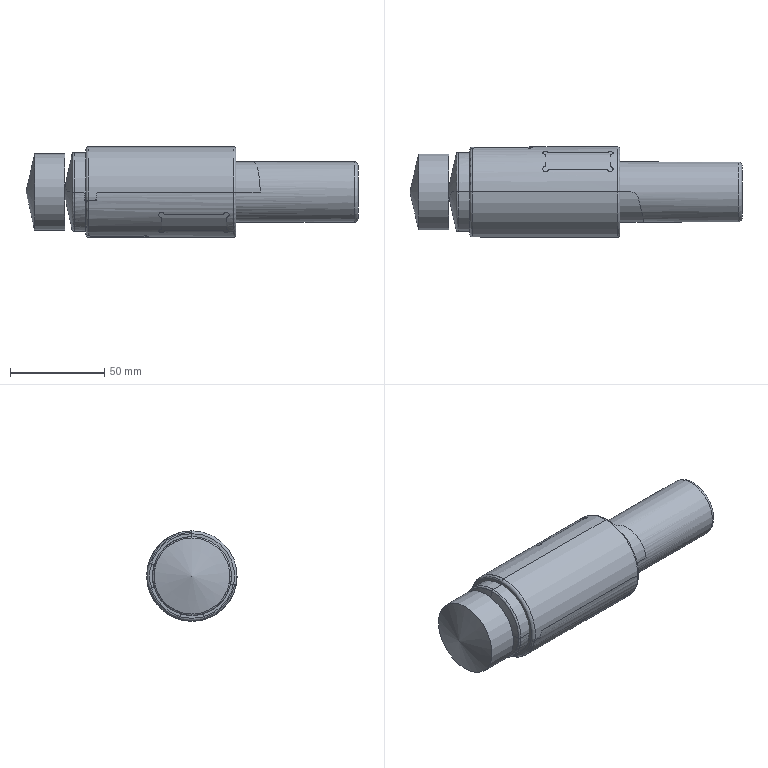NC program | NX | posted with a generic post | part box 176.413 x 48 x 48 mm
Lines 2819 to 3940 of 71815:
(ZLEVEL_PROFILE_COPY_COPY_COPY , TOOL : D6)
N5612 T06 M6
N5614 G54
N5616 G18 G0 G90 X-130.33 Z1.925 S3800 M3
N5618 G43 Y34.947 H6
N5620 Y25.5
N5622 G94 G1 X-115.85 Y24.741 F1000.
N5624 Y24.539 Z-1.925
N5626 X-128.05 Y23.9
N5628 X-140.25 F1600.
N5630 Z1.925
N5632 X-115.85
N5634 Z-1.925
N5636 X-128.05
N5638 X-133.779 Y23.8
N5640 X-140.25
N5642 Z1.925
N5644 X-115.85
N5646 Z-1.925
N5648 X-128.05
N5650 X-133.779 Y23.7
N5652 X-140.25
N5654 Z1.925
N5656 X-115.85
N5658 Z-1.925
N5660 X-128.05
N5662 X-133.779 Y23.6
N5664 X-140.25
N5666 Z1.925
N5668 X-115.85
N5670 Z-1.925
N5672 X-128.05
N5674 X-133.779 Y23.5
N5676 X-140.25
N5678 Z1.925
N5680 X-115.85
N5682 Z-1.925
N5684 X-128.05
N5686 X-133.779 Y23.4
N5688 X-140.25
N5690 Z1.925
N5692 X-115.85
N5694 Z-1.925
N5696 X-128.05
N5698 X-133.779 Y23.3
N5700 X-140.25
N5702 Z1.925
N5704 X-115.85
N5706 Z-1.925
N5708 X-128.05
N5710 X-133.779 Y23.2
N5712 X-140.25
N5714 Z1.925
N5716 X-115.85
N5718 Z-1.925
N5720 X-128.05
N5722 X-133.779 Y23.1
N5724 X-140.25
N5726 Z1.925
N5728 X-115.85
N5730 Z-1.925
N5732 X-128.05
N5734 X-133.779 Y23.
N5736 X-140.25
N5738 Z1.925
N5740 X-115.85
N5742 Z-1.925
N5744 X-128.05
N5746 X-133.779 Y22.9
N5748 X-140.25
N5750 Z1.925
N5752 X-115.85
N5754 Z-1.925
N5756 X-128.05
N5758 X-133.779 Y22.8
N5760 X-140.25
N5762 Z1.925
N5764 X-115.85
N5766 Z-1.925
N5768 X-128.05
N5770 X-133.779 Y22.7
N5772 X-140.25
N5774 Z1.925
N5776 X-115.85
N5778 Z-1.925
N5780 X-128.05
N5782 X-133.779 Y22.6
N5784 X-140.25
N5786 Z1.925
N5788 X-115.85
N5790 Z-1.925
N5792 X-128.05
N5794 X-133.779 Y22.5
N5796 X-140.25
N5798 Z1.925
N5800 X-115.85
N5802 Z-1.925
N5804 X-128.05
N5806 X-133.779 Y22.4
N5808 X-140.25
N5810 Z1.925
N5812 X-115.85
N5814 Z-1.925
N5816 X-128.05
N5818 X-133.779 Y22.3
N5820 X-140.25
N5822 Z1.925
N5824 X-115.85
N5826 Z-1.925
N5828 X-128.05
N5830 X-133.779 Y22.2
N5832 X-140.25
N5834 Z1.925
N5836 X-115.85
N5838 Z-1.925
N5840 X-128.05
N5842 X-133.779 Y22.1
N5844 X-140.25
N5846 Z1.925
N5848 X-115.85
N5850 Z-1.925
N5852 X-128.05
N5854 X-133.779 Y22.
N5856 X-140.25
N5858 Z1.925
N5860 X-115.85
N5862 Z-1.925
N5864 X-128.05
N5866 X-133.779 Y21.9
N5868 X-140.25
N5870 Z1.925
N5872 X-115.85
N5874 Z-1.925
N5876 X-128.05
N5878 X-133.779 Y21.8
N5880 X-140.25
N5882 Z1.925
N5884 X-115.85
N5886 Z-1.925
N5888 X-128.05
N5890 X-133.779 Y21.7
N5892 X-140.25
N5894 Z1.925
N5896 X-115.85
N5898 Z-1.925
N5900 X-128.05
N5902 X-133.779 Y21.6
N5904 X-140.25
N5906 Z1.925
N5908 X-115.85
N5910 Z-1.925
N5912 X-128.05
N5914 X-133.779 Y21.5
N5916 X-140.25
N5918 Z1.925
N5920 X-115.85
N5922 Z-1.925
N5924 X-128.05
N5926 X-133.779 Y21.4
N5928 X-140.25
N5930 Z1.925
N5932 X-115.85
N5934 Z-1.925
N5936 X-128.05
N5938 X-133.779 Y21.3
N5940 X-140.25
N5942 Z1.925
N5944 X-115.85
N5946 Z-1.925
N5948 X-128.05
N5950 X-133.779 Y21.2
N5952 X-140.25
N5954 Z1.925
N5956 X-115.85
N5958 Z-1.925
N5960 X-128.05
N5962 X-133.779 Y21.1
N5964 X-140.25
N5966 Z1.925
N5968 X-115.85
N5970 Z-1.925
N5972 X-128.05
N5974 X-133.779 Y21.
N5976 X-140.25
N5978 Z1.925
N5980 X-115.85
N5982 Z-1.925
N5984 X-128.05
N5986 X-133.779 Y20.9
N5988 X-140.25
N5990 Z1.925
N5992 X-115.85
N5994 Z-1.925
N5996 X-128.05
N5998 X-133.779 Y20.8
N6000 X-140.25
N6002 Z1.925
N6004 X-115.85
N6006 Z-1.925
N6008 X-128.05
N6010 X-133.779 Y20.7
N6012 X-140.25
N6014 Z1.925
N6016 X-115.85
N6018 Z-1.925
N6020 X-128.05
N6022 X-133.779 Y20.6
N6024 X-140.25
N6026 Z1.925
N6028 X-115.85
N6030 Z-1.925
N6032 X-128.05
N6034 X-133.779 Y20.5
N6036 X-140.25
N6038 Z1.925
N6040 X-115.85
N6042 Z-1.925
N6044 X-133.779
N6046 Y22.
N6048 G0 Y34.947
(ZLEVEL_PROFILE_COPY_1 , TOOL : D6)
N6050 X-147.954 Z2.204 S4000
N6052 Y34.931
N6054 Y24.899
N6056 G1 Y23.899 F1500.
N6058 X-147.781 Z2.5
N6060 G3 X-147.259 Z2.796 R0.6
N6062 G1 X-146.879 Z2.793
N6064 X-146.358 Z2.567
N6066 G2 X-143.955 Z2.729 R3.092
N6068 X-141.804 Z1.925 R3.246
N6070 G1 X-115.85
N6072 Z-1.925
N6074 X-141.881
N6076 G2 X-144.629 Z-3.652 R3.1
N6078 G1 X-144.645 Z-3.723
N6080 X-144.735 Z-3.757
N6082 X-145.035 Z-3.903
N6084 X-145.631 Z-4.254
N6086 X-145.997 Z-4.437
N6088 G2 X-147.12 Z-5.322 R4.283
N6090 G3 X-147.691 Z-5.505 R0.6
N6092 G1 X-148.003 Z-5.438
N6094 Y24.899
N6096 G0 X-147.958 Y24.8 Z2.204
N6098 G1 Y23.8
N6100 X-147.782 Z2.502
N6102 G3 X-147.259 Z2.797 R0.6
N6104 G1 X-146.879 Z2.793
N6106 X-146.358 Z2.567
N6108 G2 X-143.955 Z2.729 R3.092
N6110 X-141.804 Z1.925 R3.246
N6112 G1 X-115.85
N6114 Z-1.925
N6116 X-141.881
N6118 G2 X-144.627 Z-3.648 R3.1
N6120 G3 X-144.991 Z-3.846 R0.725
N6122 G1 X-146.106 Z-4.469
N6124 G2 X-147.167 Z-5.321 R4.085
N6126 G3 X-147.737 Z-5.51 R0.6
N6128 G1 X-148.058 Z-5.444
N6130 Y24.8
N6132 G0 X-147.961 Y24.7 Z2.198
N6134 G1 Y23.7
N6136 X-147.782 Z2.502
N6138 G3 X-147.259 Z2.797 R0.6
N6140 G1 X-146.879 Z2.793
N6142 X-146.358 Z2.567
N6144 G2 X-143.955 Z2.729 R3.093
N6146 X-141.804 Z1.925 R3.246
N6148 G1 X-115.85
N6150 Z-1.925
N6152 X-141.881
N6154 G2 X-144.627 Z-3.648 R3.1
N6156 X-146.568 Z-4.733 R16.601
N6158 G1 X-147.215 Z-5.32
N6160 G3 X-147.801 Z-5.448 R0.6
N6162 G1 X-148.052 Z-5.367
N6164 Y24.7
N6166 G0 X-147.958 Y24.6 Z2.203
N6168 G1 Y23.6
N6170 X-147.781 Z2.5
N6172 G3 X-147.257 Z2.793 R0.6
N6174 G1 X-146.861 Z2.787
N6176 X-146.358 Z2.567
N6178 G2 X-143.955 Z2.729 R3.099
N6180 X-141.804 Z1.925 R3.246
N6182 G1 X-115.85
N6184 Z-1.925
N6186 X-141.881
N6188 G2 X-144.635 Z-3.635 R3.153
N6190 X-145.929 Z-4.322 R6.532
N6192 X-147.262 Z-5.32 R4.227
N6194 G3 X-147.832 Z-5.507 R0.6
N6196 G1 X-148.154 Z-5.439
N6198 Y24.6
N6200 G0 X-147.958 Y24.5 Z2.203
N6202 G1 Y23.5
N6204 X-147.781 Z2.5
N6206 G3 X-147.257 Z2.793 R0.6
N6208 G1 X-146.861 Z2.787
N6210 X-146.358 Z2.566
N6212 G2 X-143.954 Z2.729 R3.1
N6214 X-141.804 Z1.925 R3.245
N6216 G1 X-115.85
N6218 Z-1.925
N6220 X-141.881
N6222 G2 X-144.606 Z-3.592 R3.126
N6224 X-145.957 Z-4.308 R5.848
N6226 X-147.309 Z-5.319 R4.307
N6228 G3 X-147.88 Z-5.505 R0.6
N6230 G1 X-148.203 Z-5.437
N6232 Y24.5
N6234 G0 X-147.959 Y24.401 Z2.203
N6236 G1 Y23.401
N6238 X-147.781 Z2.5
N6240 G3 X-147.257 Z2.793 R0.6
N6242 G1 X-146.861 Z2.787
N6244 X-146.358 Z2.566
N6246 G2 X-144.008 Z2.702 R3.102
N6248 G1 X-144. Z2.701
N6250 X-143.939 Z2.735
N6252 G2 X-141.85 Z1.925 R3.1
N6254 G1 X-115.85
N6256 Z-1.925
N6258 X-141.85
N6260 G2 X-144.565 Z-3.529 R3.1
N6262 G1 X-145.333 Z-3.877
N6264 G3 X-146.525 Z-4.589 R25.416
N6266 G1 X-146.625 Z-4.662
N6268 X-147.359 Z-5.321
N6270 G3 X-147.947 Z-5.444 R0.6
N6272 G1 X-148.198 Z-5.362
N6274 Y24.401
N6276 G0 X-147.957 Y24.301 Z2.201
N6278 G1 Y23.301
N6280 X-147.78 Z2.499
N6282 G3 X-147.257 Z2.792 R0.6
N6284 G1 X-146.861 Z2.787
N6286 X-146.358 Z2.566
N6288 G2 X-144.008 Z2.702 R3.104
N6290 G1 X-144. Z2.701
N6292 X-143.939 Z2.735
N6294 G2 X-141.85 Z1.925 R3.1
N6296 G1 X-115.85
N6298 Z-1.925
N6300 X-141.85
N6302 G2 X-144.546 Z-3.495 R3.1
N6304 G1 X-144.627 Z-3.47
N6306 X-144.633 Z-3.481
N6308 G2 X-145.333 Z-3.745 R1.605
N6310 G1 X-145.36 Z-3.846
N6312 X-145.84 Z-4.142
N6314 X-145.929 Z-4.184
N6316 X-145.967 Z-4.251
N6318 X-146.227 Z-4.383
N6320 G2 X-147.415 Z-5.328 R4.935
N6322 G3 X-147.987 Z-5.507 R0.6
N6324 G1 X-148.303 Z-5.437
N6326 Y24.301
N6328 G0 X-147.959 Y24.201 Z2.204
N6330 G1 Y23.201
N6332 X-147.781 Z2.501
N6334 G3 X-147.257 Z2.793 R0.6
N6336 G1 X-146.861 Z2.787
N6338 X-146.358 Z2.566
N6340 G2 X-144.008 Z2.702 R3.106
N6342 G1 X-144. Z2.701
N6344 X-143.939 Z2.735
N6346 G2 X-141.85 Z1.925 R3.1
N6348 G1 X-115.85
N6350 Z-1.925
N6352 X-141.85
N6354 G2 X-144.546 Z-3.495 R3.1
N6356 G1 X-144.628 Z-3.466
N6358 X-144.634 Z-3.478
N6360 G2 X-146.032 Z-4.092 R1.887
N6362 G1 X-145.99 Z-4.084
N6364 X-145.938 Z-4.135
N6366 X-145.972 Z-4.221
N6368 X-146.575 Z-4.534
N6370 X-146.625 Z-4.573
N6372 X-147.477 Z-5.342
N6374 G3 X-148.064 Z-5.468 R0.6
N6376 G1 X-148.315 Z-5.387
N6378 Y24.201
N6380 G0 X-147.957 Y24.101 Z2.201
N6382 G1 Y23.101
N6384 X-147.78 Z2.498
N6386 G3 X-147.257 Z2.792 R0.6
N6388 G1 X-146.861 Z2.787
N6390 X-146.358 Z2.566
N6392 G2 X-144.008 Z2.702 R3.107
N6394 G1 X-144. Z2.701
N6396 X-143.939 Z2.735
N6398 G2 X-141.85 Z1.925 R3.1
N6400 G1 X-115.85
N6402 Z-1.925
N6404 X-141.85
N6406 G2 X-144.408 Z-3.273 R3.1
N6408 X-146.575 Z-4.486 R3.059
N6410 G1 X-146.625 Z-4.515
N6412 X-147.511 Z-5.328
N6414 G3 X-148.097 Z-5.459 R0.6
N6416 G1 X-148.358 Z-5.376
N6418 Y24.101
N6420 G0 X-147.961 Y24.002 Z2.205
N6422 G1 Y23.002
N6424 X-147.781 Z2.501
N6426 G3 X-147.255 Z2.79 R0.6
N6428 G1 X-146.862 Z2.781
N6430 X-146.358 Z2.566
N6432 G2 X-144.008 Z2.702 R3.109
N6434 G1 X-144. Z2.701
N6436 X-143.939 Z2.735
N6438 G2 X-141.85 Z1.925 R3.1
N6440 G1 X-115.85
N6442 Z-1.925
N6444 X-141.85
N6446 G2 X-144.356 Z-3.2 R3.1
N6448 X-146.774 Z-4.604 R3.143
N6450 G1 X-147.575 Z-5.344
N6452 G3 X-148.16 Z-5.476 R0.6
N6454 G1 X-148.421 Z-5.395
N6456 Y24.002
N6458 G0 X-147.943 Y23.902 Z2.191
N6460 G1 Y22.902
N6462 X-147.772 Z2.484
N6464 G3 X-147.251 Z2.781 R0.6
N6466 G2 X-146.862 Z2.781 R38.615
N6468 G1 X-146.358 Z2.566
N6470 G2 X-144.007 Z2.701 R3.111
N6472 G1 X-144.
N6474 X-143.939 Z2.735
N6476 G2 X-141.85 Z1.925 R3.1
N6478 G1 X-115.85
N6480 Z-1.925
N6482 X-141.85
N6484 G2 X-144.288 Z-3.11 R3.1
N6486 G1 X-144.295 Z-3.152
N6488 X-144.367 Z-3.151
N6490 G2 X-146.823 Z-4.56 R3.132
N6492 G1 X-146.873 Z-4.633
N6494 X-146.965 Z-4.733
N6496 X-147.611 Z-5.332
N6498 G3 X-148.196 Z-5.465 R0.6
N6500 G1 X-148.462 Z-5.383
N6502 Y23.902
N6504 G0 X-147.961 Y23.802 Z2.2
N6506 G1 Y22.802
N6508 X-147.781 Z2.499
N6510 G3 X-147.255 Z2.789 R0.6
N6512 X-146.862 Z2.781 R97.442
N6514 G1 X-146.358 Z2.566
N6516 G2 X-144.007 Z2.701 R3.112
N6518 G1 X-144.
N6520 X-143.939 Z2.735
N6522 G2 X-141.85 Z1.925 R3.1
N6524 G1 X-115.85
N6526 Z-1.925
N6528 X-141.85
N6530 G2 X-144.306 Z-3.134 R3.1
N6532 G1 X-144.34 Z-3.113
N6534 X-144.539 Z-3.124
N6536 G2 X-147.014 Z-4.733 R3.155
N6538 G1 X-147.657 Z-5.331
N6540 G3 X-148.242 Z-5.464 R0.6
N6542 G1 X-148.512 Z-5.381
N6544 Y23.802
N6546 G0 X-148.195 Y23.702 Z2.204
N6548 G1 Y22.702
N6550 X-147.821 Z2.601
N6552 G3 X-147.246 Z2.773 R0.6
N6554 G2 X-146.862 Z2.781 R0.77
N6556 G1 X-146.358 Z2.566
N6558 G2 X-144.007 Z2.701 R3.114
N6560 G1 X-144.
N6562 X-143.939 Z2.735
N6564 G2 X-141.85 Z1.925 R3.1
N6566 G1 X-115.85
N6568 Z-1.925
N6570 X-141.85
N6572 G2 X-144.273 Z-3.092 R3.1
N6574 X-146.659 Z-4.142 R2.949
N6576 G1 X-146.724 Z-4.23
N6578 X-146.774 Z-4.277
N6580 X-147.063 Z-4.733
N6582 X-147.704 Z-5.329
N6584 G3 X-148.288 Z-5.463 R0.6
N6586 G1 X-148.562 Z-5.38
N6588 Y23.702
N6590 G0 X-147.947 Y23.603 Z2.2
N6592 G1 Y22.603
N6594 X-147.767 Z2.478
N6596 G3 X-147.233 Z2.751 R0.6
N6598 G2 X-146.862 Z2.781 R1.437
N6600 G1 X-146.358 Z2.565
N6602 G2 X-144.007 Z2.701 R3.111
N6604 G1 X-144. Z2.7
N6606 X-143.939 Z2.735
N6608 G2 X-141.85 Z1.925 R3.1
N6610 G1 X-115.85
N6612 Z-1.925
N6614 X-141.85
N6616 G2 X-144.24 Z-3.051 R3.1
N6618 X-147.112 Z-4.733 R3.121
N6620 G1 X-147.74 Z-5.318
N6622 G3 X-148.325 Z-5.452 R0.6
N6624 G1 X-148.601 Z-5.367
N6626 Y23.603
N6628 G0 X-147.91 Y23.503 Z2.195
N6630 G1 Y22.503
N6632 X-147.752 Z2.451
N6634 G3 X-147.224 Z2.736 R0.6
N6636 G2 X-146.862 Z2.78 R1.228
N6638 G1 X-146.358 Z2.565
N6640 G2 X-144.007 Z2.701 R3.113
N6642 G1 X-144. Z2.7
N6644 X-143.939 Z2.735
N6646 G2 X-141.85 Z1.925 R3.1
N6648 G1 X-115.85
N6650 Z-1.925
N6652 X-141.85
N6654 G2 X-144.23 Z-3.039 R3.1
N6656 X-146.796 Z-4.182 R3.074
N6658 G1 X-146.821 Z-4.223
N6660 X-146.794 Z-4.237
N6662 X-146.823 Z-4.216
N6664 X-147.16 Z-4.733
N6666 X-147.788 Z-5.318
N6668 G3 X-148.372 Z-5.452 R0.6
N6670 G1 X-148.651 Z-5.367
N6672 Y23.503
N6674 G0 X-147.845 Y23.403 Z2.198
N6676 G1 Y22.403
N6678 X-147.729 Z2.412
N6680 G3 X-147.219 Z2.727 R0.6
N6682 G2 X-146.862 Z2.78 R1.51
N6684 G1 X-146.358 Z2.565
N6686 G2 X-144.007 Z2.701 R3.113
N6688 G1 X-144. Z2.7
N6690 X-143.939 Z2.735
N6692 G2 X-141.85 Z1.925 R3.1
N6694 G1 X-115.85
N6696 Z-1.925
N6698 X-141.85
N6700 G2 X-144.202 Z-3.006 R3.1
N6702 X-147.022 Z-4.443 R3.127
N6704 G1 X-147.121 Z-4.611
N6706 X-147.208 Z-4.733
N6708 X-147.831 Z-5.314
N6710 G3 X-148.416 Z-5.448 R0.6
N6712 G1 X-148.697 Z-5.362
N6714 Y23.403
N6716 G0 X-147.818 Y23.303 Z2.172
N6718 G1 Y22.303
N6720 X-147.713 Z2.385
N6722 G3 X-147.213 Z2.718 R0.6
N6724 G2 X-146.862 Z2.78 R1.608
N6726 G1 X-146.358 Z2.565
N6728 G2 X-144.007 Z2.701 R3.113
N6730 G1 X-144. Z2.7
N6732 X-143.939 Z2.735
N6734 G2 X-141.85 Z1.925 R3.1
N6736 G1 X-115.85
N6738 Z-1.925
N6740 X-141.85
N6742 G2 X-144.194 Z-2.997 R3.1
N6744 X-146.955 Z-4.315 R3.036
N6746 G3 X-147.835 Z-5.277 R4.571
N6748 X-148.427 Z-5.375 R0.6
N6750 G1 X-148.681 Z-5.279
N6752 Y23.303
N6754 G0 X-147.795 Y23.204 Z2.145
N6756 G1 Y22.204
N6758 X-147.701 Z2.371
N6760 G3 X-147.224 Z2.735 R0.6
N6762 G1 X-146.862 Z2.78
N6764 X-146.358 Z2.565
N6766 G2 X-144.006 Z2.701 R3.114
N6768 G1 X-144. Z2.7
N6770 X-143.939 Z2.735
N6772 G2 X-141.85 Z1.925 R3.1
N6774 G1 X-115.85
N6776 Z-1.925
N6778 X-141.85
N6780 G2 X-144.173 Z-2.973 R3.1
N6782 X-147.001 Z-4.32 R3.112
N6784 G3 X-147.838 Z-5.242 R4.509
N6786 X-148.429 Z-5.344 R0.6
N6788 G1 X-148.701 Z-5.244
N6790 Y23.204
N6792 G0 X-147.812 Y23.104 Z2.115
N6794 G1 Y22.104
N6796 X-147.703 Z2.374
N6798 G3 X-147.224 Z2.735 R0.6
N6800 G1 X-146.862 Z2.78
N6802 X-146.358 Z2.565
N6804 G2 X-144.006 Z2.7 R3.114
N6806 G1 X-144.
N6808 X-143.939 Z2.735
N6810 G2 X-141.85 Z1.925 R3.1
N6812 G1 X-115.85
N6814 Z-1.925
N6816 X-141.85
N6818 G2 X-144.141 Z-2.937 R3.1
N6820 X-147.121 Z-4.423 R3.23
N6822 G1 X-147.192 Z-4.536
N6824 G3 X-147.842 Z-5.197 R7.271
N6826 X-148.429 Z-5.321 R0.6
N6828 G1 X-148.731 Z-5.222
N6830 Y23.104
N6832 G0 X-147.826 Y23.004 Z2.08
N6834 G1 Y22.004
N6836 X-147.702 Z2.373
N6838 G3 X-147.224 Z2.735 R0.6
N6840 G1 X-146.863 Z2.78
N6842 X-146.358 Z2.565
N6844 G2 X-144.006 Z2.7 R3.113
N6846 G1 X-144.
N6848 X-143.939 Z2.735
N6850 G2 X-141.85 Z1.925 R3.1
N6852 G1 X-115.85
N6854 Z-1.925
N6856 X-141.85
N6858 G2 X-144.149 Z-2.946 R3.1
N6860 G1 X-144.173 Z-2.92
N6862 X-144.34 Z-2.904
N6864 G2 X-146.468 Z-3.649 R3.145
N6866 X-147.148 Z-4.408 R4.027
N6868 G1 X-147.23 Z-4.536
N6870 G3 X-147.844 Z-5.154 R9.349
N6872 X-148.43 Z-5.284 R0.6
N6874 G1 X-148.747 Z-5.184
N6876 Y23.004
N6878 G0 X-147.834 Y22.904 Z2.063
N6880 G1 Y21.904
N6882 X-147.703 Z2.374
N6884 G3 X-147.224 Z2.735 R0.6
N6886 G1 X-146.863 Z2.78
N6888 X-146.358 Z2.565
N6890 G2 X-144. Z2.7 R3.113
N6892 G1 X-143.939 Z2.735
N6894 G2 X-141.85 Z1.925 R3.1
N6896 G1 X-115.85
N6898 Z-1.925
N6900 X-141.85
N6902 G2 X-144.129 Z-2.924 R3.1
N6904 G1 X-144.173 Z-2.892
N6906 X-144.539 Z-2.873
N6908 G2 X-147.268 Z-4.536 R3.348
N6910 G1 X-147.847 Z-5.097
N6912 G3 X-148.429 Z-5.243 R0.6
N6914 G1 X-148.763 Z-5.148
N6916 Y22.904
N6918 G0 X-147.836 Y22.805 Z2.059
N6920 G1 Y21.805
N6922 X-147.703 Z2.374
N6924 G3 X-147.224 Z2.735 R0.6
N6926 G1 X-146.863 Z2.78
N6928 X-146.358 Z2.564
N6930 G2 X-144. Z2.7 R3.109
N6932 G1 X-143.939 Z2.735
N6934 G2 X-141.85 Z1.925 R3.1
N6936 G1 X-115.85
N6938 Z-1.925
N6940 X-141.85
N6942 G2 X-144.115 Z-2.909 R3.1
N6944 G1 X-144.141 Z-2.879
N6946 X-144.539 Z-2.843
N6948 G2 X-147.305 Z-4.536 R3.31
N6950 G1 X-147.848 Z-5.055
N6952 G3 X-148.431 Z-5.197 R0.6
N6954 G1 X-148.766 Z-5.099
N6956 Y22.805
N6958 G0 X-147.804 Y22.705 Z2.063
N6960 G1 Y21.705
N6962 X-147.688 Z2.351
N6964 G3 X-147.215 Z2.72 R0.6
N6966 G2 X-146.863 Z2.78 R6.744
N6968 G1 X-146.358 Z2.564
N6970 G2 X-144. Z2.7 R3.105
N6972 G1 X-143.939 Z2.735
N6974 G2 X-141.85 Z1.925 R3.1
N6976 G1 X-115.85
N6978 Z-1.925
N6980 X-141.85
N6982 G2 X-144.078 Z-2.87 R3.1
N6984 G1 X-144.174 Z-2.835
N6986 X-144.737 Z-2.821
N6988 G2 X-147.343 Z-4.536 R3.265
N6990 G1 X-147.849 Z-5.014
N6992 G3 X-148.433 Z-5.152 R0.6
N6994 G1 X-148.769 Z-5.052
N6996 Y22.705
N6998 G0 X-147.844 Y22.605 Z2.041
N7000 G1 Y21.605
N7002 X-147.703 Z2.374
N7004 G3 X-147.224 Z2.735 R0.6
N7006 G1 X-146.863 Z2.78
N7008 X-146.358 Z2.564
N7010 G2 X-144. Z2.699 R3.105
N7012 G1 X-143.939 Z2.735
N7014 G2 X-141.85 Z1.925 R3.1
N7016 G1 X-115.85
N7018 Z-1.925
N7020 X-141.85
N7022 G2 X-144.063 Z-2.854 R3.1
N7024 G1 X-144.085 Z-2.828
N7026 X-144.539 Z-2.784
N7028 G2 X-147.381 Z-4.536 R3.232
N7030 G1 X-147.849 Z-4.973
N7032 G3 X-148.434 Z-5.108 R0.6
N7034 G1 X-148.769 Z-5.005
N7036 Y22.605
N7038 G0 X-147.815 Y22.506 Z2.058
N7040 G1 Y21.506
N7042 X-147.692 Z2.358
N7044 G3 X-147.218 Z2.725 R0.6
N7046 G2 X-146.863 Z2.779 R11.412
N7048 G1 X-146.358 Z2.564
N7050 G2 X-144. Z2.699 R3.1
N7052 G1 X-143.939 Z2.735
N7054 G2 X-141.85 Z1.925 R3.1
N7056 G1 X-115.85
N7058 Z-1.925
N7060 X-141.85
N7062 G2 X-144.028 Z-2.819 R3.1
N7064 X-147.18 Z-4.142 R3.047
N7066 G1 X-147.427 Z-4.536
N7068 X-147.849 Z-4.928
N7070 G3 X-148.434 Z-5.063 R0.6
N7072 G1 X-148.77 Z-4.959
N7074 Y22.506
N7076 G0 X-147.828 Y22.406 Z2.05
N7078 G1 Y21.406
N7080 X-147.697 Z2.366
N7082 G3 X-147.221 Z2.731 R0.6
N7084 G2 X-146.863 Z2.779 R55.903
N7086 G1 X-146.358 Z2.564
N7088 G2 X-144. Z2.699 R3.099
N7090 G1 X-143.939 Z2.735
N7092 G2 X-141.85 Z1.925 R3.1
N7094 G1 X-115.85
N7096 Z-1.925
N7098 X-141.85
N7100 G2 X-143.999 Z-2.791 R3.1
N7102 X-147.23 Z-4.142 R3.058
N7104 G1 X-147.474 Z-4.536
N7106 X-147.848 Z-4.883
N7108 G3 X-148.432 Z-5.017 R0.6
N7110 G1 X-148.77 Z-4.913
N7112 Y22.406
N7114 G0 X-147.823 Y22.306 Z2.052
N7116 G1 Y21.306
N7118 X-147.695 Z2.363
N7120 G3 X-147.22 Z2.729 R0.6
N7122 G2 X-146.863 Z2.779 R26.17
N7124 G1 X-146.358 Z2.564
N7126 G2 X-144. Z2.699 R3.094
N7128 G1 X-143.939 Z2.735
N7130 G2 X-141.85 Z1.925 R3.1
N7132 G1 X-115.85
N7134 Z-1.925
N7136 X-141.85
N7138 G2 X-143.942 Z-2.737 R3.1
N7140 G1 X-143.979 Z-2.754
N7142 X-144.141 Z-2.722
N7144 G2 X-147.414 Z-4.385 R3.093
N7146 G1 X-147.521 Z-4.536
N7148 X-147.846 Z-4.837
N7150 G3 X-148.431 Z-4.971 R0.6
N7152 G1 X-148.763 Z-4.869
N7154 Y22.306
N7156 G0 X-147.827 Y22.206 Z2.05
N7158 G1 Y21.206
N7160 X-147.697 Z2.365
N7162 G3 X-147.221 Z2.73 R0.6
N7164 G2 X-146.863 Z2.779 R46.907
N7166 G1 X-146.334 Z2.555
N7168 G2 X-144. Z2.699 R3.088
N7170 G1 X-143.939 Z2.735
N7172 G2 X-141.85 Z1.925 R3.1
N7174 G1 X-115.85
N7176 Z-1.925
N7178 X-141.85
N7180 G2 X-143.94 Z-2.735 R3.1
N7182 X-147.457 Z-4.381 R3.086
N7184 G1 X-147.568 Z-4.536
N7186 X-147.844 Z-4.791
N7188 G3 X-148.429 Z-4.924 R0.6
N7190 G1 X-148.76 Z-4.822
N7192 Y22.206
N7194 G0 X-147.828 Y22.107 Z2.049
N7196 G1 Y21.107
N7198 X-147.697 Z2.365
N7200 G3 X-147.221 Z2.731 R0.6
N7202 G2 X-146.863 Z2.779 R64.992
N7204 G1 X-146.334 Z2.555
N7206 G2 X-144.029 Z2.686 R3.09
N7208 G1 X-143.898 Z2.698
N7210 G2 X-141.85 Z1.925 R3.1
N7212 G1 X-115.85
N7214 Z-1.925
N7216 X-141.85
N7218 G2 X-143.908 Z-2.707 R3.1
N7220 G3 X-144.331 Z-2.281 R0.6
N7222 G1 X-144.402 Z-2.013
N7224 Y22.107
N7226 G0 Y34.942
N7228 X-145.632 Y34.921 Z-2.357
N7230 X-146.862 Y34.896 Z-2.701
N7232 Y22.107
N7234 G1 Y21.107
N7236 X-146.784 Z-2.966
N7238 G3 X-146.924 Z-3.55 R0.6
N7240 G1 X-147.015 Z-3.647
N7242 X-147.428 Z-4.238
N7244 X-147.616 Z-4.536
N7246 X-147.717 Z-4.625
N7248 X-147.841 Z-4.74
N7250 G3 X-148.425 Z-4.875 R0.6
N7252 G1 X-148.757 Z-4.774
N7254 Y22.107
N7256 G0 Y34.673
(ZLEVEL_PROFILE_COPY_COPY_COPY_COPY , TOOL : D6)
N7258 G17 X-130.33 Y1.925 S3800
N7260 Z-34.947
N7262 Z-25.5
N7264 G1 X-115.85 Z-24.741 F1000.
N7266 Y-1.925 Z-24.539
N7268 X-128.05 Z-23.9
N7270 X-140.25 F1600.
N7272 Y1.925
N7274 X-115.85
N7276 Y-1.925
N7278 X-128.05
N7280 X-133.779 Z-23.8
N7282 X-140.25
N7284 Y1.925
N7286 X-115.85
N7288 Y-1.925
N7290 X-128.05
N7292 X-133.779 Z-23.7
N7294 X-140.25
N7296 Y1.925
N7298 X-115.85
N7300 Y-1.925
N7302 X-128.05
N7304 X-133.779 Z-23.6
N7306 X-140.25
N7308 Y1.925
N7310 X-115.85
N7312 Y-1.925
N7314 X-128.05
N7316 X-133.779 Z-23.5
N7318 X-140.25
N7320 Y1.925
N7322 X-115.85
N7324 Y-1.925
N7326 X-128.05
N7328 X-133.779 Z-23.4
N7330 X-140.25
N7332 Y1.925
N7334 X-115.85
N7336 Y-1.925
N7338 X-128.05
N7340 X-133.779 Z-23.3
N7342 X-140.25
N7344 Y1.925
N7346 X-115.85
N7348 Y-1.925
N7350 X-128.05
N7352 X-133.779 Z-23.2
N7354 X-140.25
N7356 Y1.925
N7358 X-115.85
N7360 Y-1.925
N7362 X-128.05
N7364 X-133.779 Z-23.1
N7366 X-140.25
N7368 Y1.925
N7370 X-115.85
N7372 Y-1.925
N7374 X-128.05
N7376 X-133.779 Z-23.
N7378 X-140.25
N7380 Y1.925
N7382 X-115.85
N7384 Y-1.925
N7386 X-128.05
N7388 X-133.779 Z-22.9
N7390 X-140.25
N7392 Y1.925
N7394 X-115.85
N7396 Y-1.925
N7398 X-128.05
N7400 X-133.779 Z-22.8
N7402 X-140.25
N7404 Y1.925
N7406 X-115.85
N7408 Y-1.925
N7410 X-128.05
N7412 X-133.779 Z-22.7
N7414 X-140.25
N7416 Y1.925
N7418 X-115.85
N7420 Y-1.925
N7422 X-128.05
N7424 X-133.779 Z-22.6
N7426 X-140.25
N7428 Y1.925
N7430 X-115.85
N7432 Y-1.925
N7434 X-128.05
N7436 X-133.779 Z-22.5
N7438 X-140.25
N7440 Y1.925
N7442 X-115.85
N7444 Y-1.925
N7446 X-128.05
N7448 X-133.779 Z-22.4
N7450 X-140.25
N7452 Y1.925
N7454 X-115.85
N7456 Y-1.925
N7458 X-128.05
N7460 X-133.779 Z-22.3
N7462 X-140.25
N7464 Y1.925
N7466 X-115.85
N7468 Y-1.925
N7470 X-128.05
N7472 X-133.779 Z-22.2
N7474 X-140.25
N7476 Y1.925
N7478 X-115.85
N7480 Y-1.925
N7482 X-128.05
N7484 X-133.779 Z-22.1
N7486 X-140.25
N7488 Y1.925
N7490 X-115.85
N7492 Y-1.925
N7494 X-128.05
N7496 X-133.779 Z-22.
N7498 X-140.25
N7500 Y1.925
N7502 X-115.85
N7504 Y-1.925
N7506 X-128.05
N7508 X-133.779 Z-21.9
N7510 X-140.25
N7512 Y1.925
N7514 X-115.85
N7516 Y-1.925
N7518 X-128.05
N7520 X-133.779 Z-21.8
N7522 X-140.25
N7524 Y1.925
N7526 X-115.85
N7528 Y-1.925
N7530 X-128.05
N7532 X-133.779 Z-21.7
N7534 X-140.25
N7536 Y1.925
N7538 X-115.85
N7540 Y-1.925
N7542 X-128.05
N7544 X-133.779 Z-21.6
N7546 X-140.25
N7548 Y1.925
N7550 X-115.85
N7552 Y-1.925
N7554 X-128.05
N7556 X-133.779 Z-21.5
N7558 X-140.25
N7560 Y1.925
N7562 X-115.85
N7564 Y-1.925
N7566 X-128.05
N7568 X-133.779 Z-21.4
N7570 X-140.25
N7572 Y1.925
N7574 X-115.85
N7576 Y-1.925
N7578 X-128.05
N7580 X-133.779 Z-21.3
N7582 X-140.25
N7584 Y1.925
N7586 X-115.85
N7588 Y-1.925
N7590 X-128.05
N7592 X-133.779 Z-21.2
N7594 X-140.25
N7596 Y1.925
N7598 X-115.85
N7600 Y-1.925
N7602 X-128.05
N7604 X-133.779 Z-21.1
N7606 X-140.25
N7608 Y1.925
N7610 X-115.85
N7612 Y-1.925
N7614 X-128.05
N7616 X-133.779 Z-21.
N7618 X-140.25
N7620 Y1.925
N7622 X-115.85
N7624 Y-1.925
N7626 X-128.05
N7628 X-133.779 Z-20.9
N7630 X-140.25
N7632 Y1.925
N7634 X-115.85
N7636 Y-1.925
N7638 X-128.05
N7640 X-133.779 Z-20.8
N7642 X-140.25
N7644 Y1.925
N7646 X-115.85
N7648 Y-1.925
N7650 X-128.05
N7652 X-133.779 Z-20.7
N7654 X-140.25
N7656 Y1.925
N7658 X-115.85
N7660 Y-1.925
N7662 X-128.05
N7664 X-133.779 Z-20.6
N7666 X-140.25
N7668 Y1.925
N7670 X-115.85
N7672 Y-1.925
N7674 X-128.05
N7676 X-133.779 Z-20.5
N7678 X-140.25
N7680 Y1.925
N7682 X-115.85
N7684 Y-1.925
N7686 X-133.779
N7688 Z-22.
N7690 G0 Z-34.947
(ZLEVEL_PROFILE_COPY_1_COPY , TOOL : D6)
N7692 Z-34.931 S4000
N7694 X-147.954 Y2.204
N7696 Z-24.899
N7698 G1 Z-23.899 F1500.
N7700 X-147.781 Y2.5
N7702 G2 X-147.259 Y2.796 R0.6
N7704 G1 X-146.879 Y2.793
N7706 X-146.358 Y2.567
N7708 G3 X-143.955 Y2.729 R3.092
N7710 X-141.804 Y1.925 R3.246
N7712 G1 X-115.85
N7714 Y-1.925
N7716 X-141.881
N7718 G3 X-144.629 Y-3.652 R3.1
N7720 G1 X-144.652 Y-3.734
N7722 X-144.735 Y-3.757
N7724 X-145.035 Y-3.903
N7726 X-145.631 Y-4.254
N7728 X-145.997 Y-4.437
N7730 G3 X-147.12 Y-5.322 R4.283
N7732 G2 X-147.691 Y-5.505 R0.6
N7734 G1 X-148.003 Y-5.438
N7736 Z-24.899
N7738 G0 X-147.958 Y2.204 Z-24.8
N7740 G1 Z-23.8
N7742 X-147.782 Y2.502
N7744 G2 X-147.259 Y2.797 R0.6
N7746 G1 X-146.879 Y2.793
N7748 X-146.358 Y2.567
N7750 G3 X-143.955 Y2.729 R3.092
N7752 X-141.804 Y1.925 R3.246
N7754 G1 X-115.85
N7756 Y-1.925
N7758 X-141.881
N7760 G3 X-144.627 Y-3.648 R3.1
N7762 G2 X-144.991 Y-3.846 R0.725
N7764 G1 X-146.106 Y-4.469
N7766 G3 X-147.167 Y-5.321 R4.085
N7768 G2 X-147.737 Y-5.51 R0.6
N7770 G1 X-148.058 Y-5.444
N7772 Z-24.8
N7774 G0 X-147.961 Y2.198 Z-24.7
N7776 G1 Z-23.7
N7778 X-147.782 Y2.502
N7780 G2 X-147.259 Y2.797 R0.6
N7782 G1 X-146.879 Y2.793
N7784 X-146.358 Y2.567
N7786 G3 X-143.955 Y2.729 R3.093
N7788 X-141.804 Y1.925 R3.246
N7790 G1 X-115.85
N7792 Y-1.925
N7794 X-141.881
N7796 G3 X-144.627 Y-3.648 R3.1
N7798 X-146.568 Y-4.733 R16.601
N7800 G1 X-147.215 Y-5.32
N7802 G2 X-147.801 Y-5.448 R0.6
N7804 G1 X-148.052 Y-5.367
N7806 Z-24.7
N7808 G0 X-147.958 Y2.203 Z-24.6
N7810 G1 Z-23.6
N7812 X-147.781 Y2.5
N7814 G2 X-147.257 Y2.793 R0.6
N7816 G1 X-146.861 Y2.787
N7818 X-146.358 Y2.567
N7820 G3 X-143.955 Y2.729 R3.099
N7822 X-141.804 Y1.925 R3.246
N7824 G1 X-115.85
N7826 Y-1.925
N7828 X-141.881
N7830 G3 X-144.635 Y-3.635 R3.153